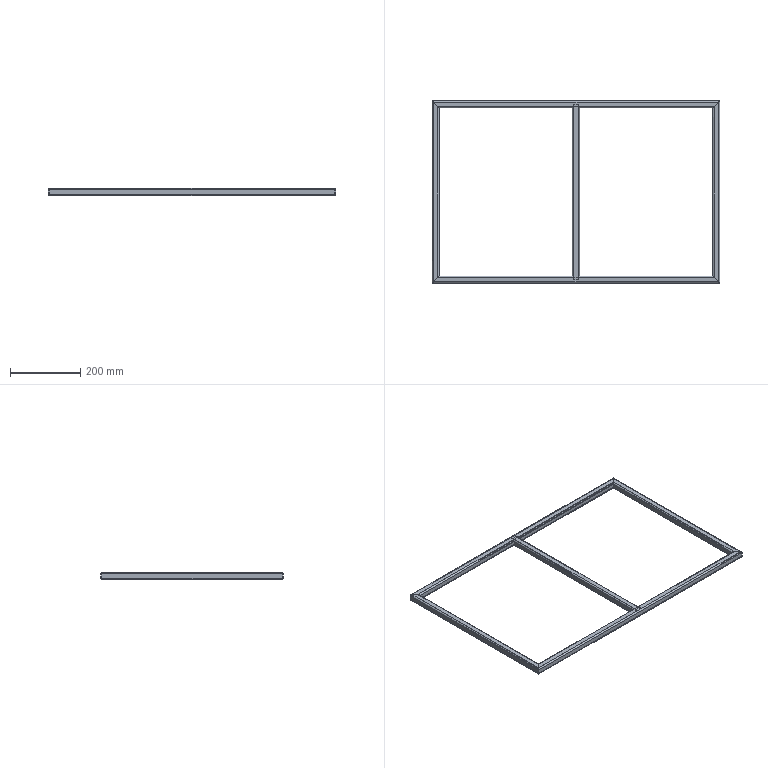Part | SolidWorks | features WeldMemberFeat 2, WeldmentFeature 1 | 5 solids | 90 faces | box 820 x 520 x 20 mm | volume 414467 mm3 | plane 50 | cylinder 40 | commonest cylinder face diameters 4 x20 8 x20